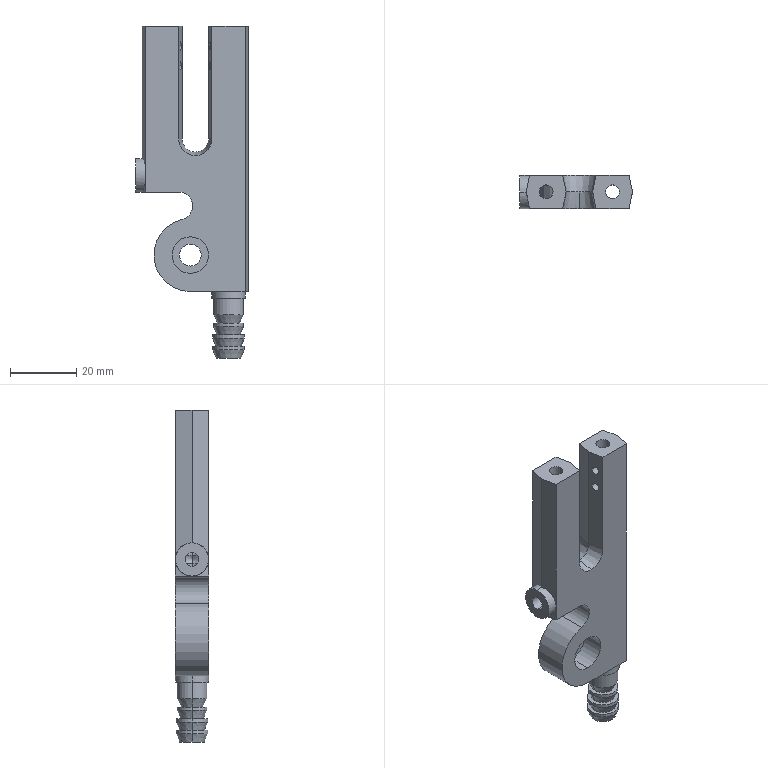Part | SolidWorks | features MBimport 1 | 1 solid | 85 faces | box 34 x 10 x 100 mm | volume 16950 mm3 | cylinder 40 | plane 24 | cone 21 | commonest cylinder face diameters 4.2 x12 2.5 x8 9.5 x4 10 x4 5 x2 6.6 x2